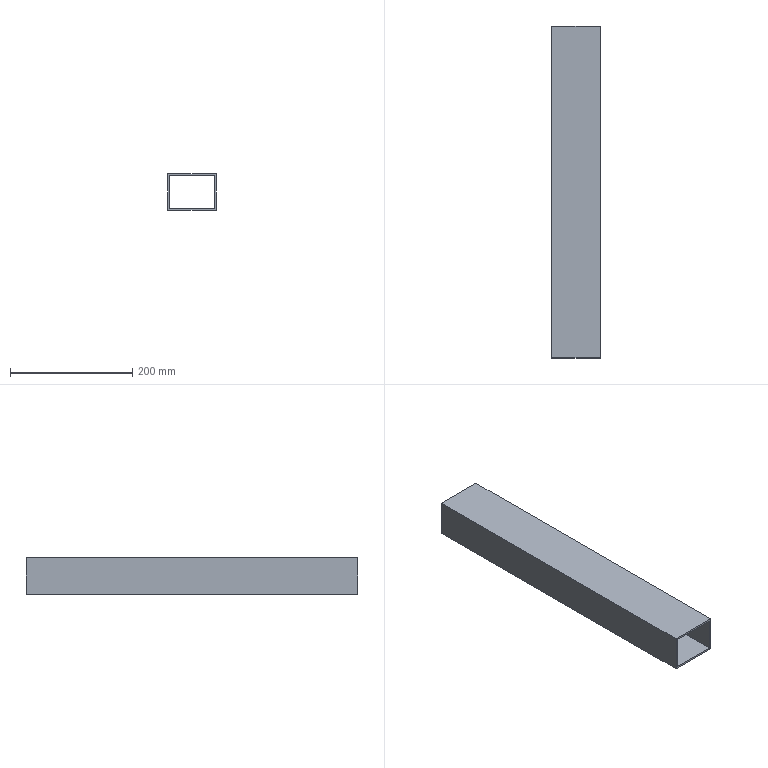Part | STEP file | Guide wheel mechanism revised.sldasm-Part-26 | 1 solid | 10 faces | box 80 x 541.99 x 60 mm | volume 435760 mm3 | plane 10
STEP:
#1=CARTESIAN_POINT('',(405.,1970.,445.));
#2=VERTEX_POINT('',#1);
#3=CARTESIAN_POINT('',(405.,1428.01,445.));
#4=VERTEX_POINT('',#3);
#5=CARTESIAN_POINT('',(405.,1970.,445.));
#6=DIRECTION('',(0.,-1.,0.));
#7=VECTOR('',#6,1000.);
#8=LINE('',#5,#7);
#9=EDGE_CURVE('',#2,#4,#8,.T.);
#10=ORIENTED_EDGE('',*,*,#9,.T.);
#11=CARTESIAN_POINT('',(405.,1428.01,505.));
#12=VERTEX_POINT('',#11);
#13=CARTESIAN_POINT('',(405.,1428.01,-160.471));
#14=DIRECTION('',(0.,0.,1.));
#15=VECTOR('',#14,1000.);
#16=LINE('',#13,#15);
#17=EDGE_CURVE('',#4,#12,#16,.T.);
#18=ORIENTED_EDGE('',*,*,#17,.T.);
#19=CARTESIAN_POINT('',(405.,1970.,505.));
#20=VERTEX_POINT('',#19);
#21=CARTESIAN_POINT('',(405.,1970.,505.));
#22=DIRECTION('',(0.,-1.,0.));
#23=VECTOR('',#22,1000.);
#24=LINE('',#21,#23);
#25=EDGE_CURVE('',#20,#12,#24,.T.);
#26=ORIENTED_EDGE('',*,*,#25,.F.);
#27=CARTESIAN_POINT('',(405.,1970.,505.));
#28=DIRECTION('',(0.,0.,1.));
#29=VECTOR('',#28,1000.);
#30=LINE('',#27,#29);
#31=EDGE_CURVE('',#2,#20,#30,.T.);
#32=ORIENTED_EDGE('',*,*,#31,.F.);
#33=EDGE_LOOP('',(#10,#18,#26,#32));
#34=FACE_OUTER_BOUND('',#33,.T.);
#35=CARTESIAN_POINT('',(405.,1970.,505.));
#36=DIRECTION('',(1.,0.,0.));
#37=DIRECTION('',(0.,0.,-1.));
#38=AXIS2_PLACEMENT_3D('',#35,#36,#37);
#39=PLANE('',#38);
#40=ADVANCED_FACE('',(#34),#39,.F.);
#41=ORIENTED_EDGE('',*,*,#25,.T.);
#42=CARTESIAN_POINT('',(485.,1428.01,505.));
#43=VERTEX_POINT('',#42);
#44=CARTESIAN_POINT('',(405.,1428.01,505.));
#45=DIRECTION('',(-1.,0.,0.));
#46=VECTOR('',#45,1000.);
#47=LINE('',#44,#46);
#48=EDGE_CURVE('',#43,#12,#47,.T.);
#49=ORIENTED_EDGE('',*,*,#48,.F.);
#50=CARTESIAN_POINT('',(485.,1970.,505.));
#51=VERTEX_POINT('',#50);
#52=CARTESIAN_POINT('',(485.,1970.,505.));
#53=DIRECTION('',(0.,-1.,0.));
#54=VECTOR('',#53,1000.);
#55=LINE('',#52,#54);
#56=EDGE_CURVE('',#51,#43,#55,.T.);
#57=ORIENTED_EDGE('',*,*,#56,.F.);
#58=CARTESIAN_POINT('',(485.,1970.,505.));
#59=DIRECTION('',(1.,0.,0.));
#60=VECTOR('',#59,1000.);
#61=LINE('',#58,#60);
#62=EDGE_CURVE('',#20,#51,#61,.T.);
#63=ORIENTED_EDGE('',*,*,#62,.F.);
#64=EDGE_LOOP('',(#41,#49,#57,#63));
#65=FACE_OUTER_BOUND('',#64,.T.);
#66=CARTESIAN_POINT('',(485.,1970.,505.));
#67=DIRECTION('',(0.,0.,-1.));
#68=DIRECTION('',(-1.,0.,0.));
#69=AXIS2_PLACEMENT_3D('',#66,#67,#68);
#70=PLANE('',#69);
#71=ADVANCED_FACE('',(#65),#70,.F.);
#72=ORIENTED_EDGE('',*,*,#56,.T.);
#73=CARTESIAN_POINT('',(485.,1428.01,445.));
#74=VERTEX_POINT('',#73);
#75=CARTESIAN_POINT('',(485.,1428.01,505.));
#76=DIRECTION('',(0.,0.,-1.));
#77=VECTOR('',#76,1000.);
#78=LINE('',#75,#77);
#79=EDGE_CURVE('',#43,#74,#78,.T.);
#80=ORIENTED_EDGE('',*,*,#79,.T.);
#81=CARTESIAN_POINT('',(485.,1970.,445.));
#82=VERTEX_POINT('',#81);
#83=CARTESIAN_POINT('',(485.,1970.,445.));
#84=DIRECTION('',(0.,-1.,0.));
#85=VECTOR('',#84,1000.);
#86=LINE('',#83,#85);
#87=EDGE_CURVE('',#82,#74,#86,.T.);
#88=ORIENTED_EDGE('',*,*,#87,.F.);
#89=CARTESIAN_POINT('',(485.,1970.,505.));
#90=DIRECTION('',(0.,0.,-1.));
#91=VECTOR('',#90,1000.);
#92=LINE('',#89,#91);
#93=EDGE_CURVE('',#51,#82,#92,.T.);
#94=ORIENTED_EDGE('',*,*,#93,.F.);
#95=EDGE_LOOP('',(#72,#80,#88,#94));
#96=FACE_OUTER_BOUND('',#95,.T.);
#97=CARTESIAN_POINT('',(485.,1970.,505.));
#98=DIRECTION('',(-1.,0.,0.));
#99=DIRECTION('',(0.,0.,1.));
#100=AXIS2_PLACEMENT_3D('',#97,#98,#99);
#101=PLANE('',#100);
#102=ADVANCED_FACE('',(#96),#101,.F.);
#103=ORIENTED_EDGE('',*,*,#87,.T.);
#104=CARTESIAN_POINT('',(405.,1428.01,445.));
#105=DIRECTION('',(1.,0.,0.));
#106=VECTOR('',#105,1000.);
#107=LINE('',#104,#106);
#108=EDGE_CURVE('',#4,#74,#107,.T.);
#109=ORIENTED_EDGE('',*,*,#108,.F.);
#110=ORIENTED_EDGE('',*,*,#9,.F.);
#111=CARTESIAN_POINT('',(485.,1970.,445.));
#112=DIRECTION('',(-1.,0.,0.));
#113=VECTOR('',#112,1000.);
#114=LINE('',#111,#113);
#115=EDGE_CURVE('',#82,#2,#114,.T.);
#116=ORIENTED_EDGE('',*,*,#115,.F.);
#117=EDGE_LOOP('',(#103,#109,#110,#116));
#118=FACE_OUTER_BOUND('',#117,.T.);
#119=CARTESIAN_POINT('',(485.,1970.,445.));
#120=DIRECTION('',(0.,0.,1.));
#121=DIRECTION('',(1.,0.,0.));
#122=AXIS2_PLACEMENT_3D('',#119,#120,#121);
#123=PLANE('',#122);
#124=ADVANCED_FACE('',(#118),#123,.F.);
#125=CARTESIAN_POINT('',(482.,1428.01,502.));
#126=VERTEX_POINT('',#125);
#127=CARTESIAN_POINT('',(482.,1428.01,448.));
#128=VERTEX_POINT('',#127);
#129=CARTESIAN_POINT('',(482.,1428.01,502.));
#130=DIRECTION('',(0.,0.,-1.));
#131=VECTOR('',#130,1000.);
#132=LINE('',#129,#131);
#133=EDGE_CURVE('',#126,#128,#132,.T.);
#134=ORIENTED_EDGE('',*,*,#133,.F.);
#135=CARTESIAN_POINT('',(482.,1970.,502.));
#136=VERTEX_POINT('',#135);
#137=CARTESIAN_POINT('',(482.,1970.,502.));
#138=DIRECTION('',(0.,-1.,0.));
#139=VECTOR('',#138,1000.);
#140=LINE('',#137,#139);
#141=EDGE_CURVE('',#136,#126,#140,.T.);
#142=ORIENTED_EDGE('',*,*,#141,.F.);
#143=CARTESIAN_POINT('',(482.,1970.,448.));
#144=VERTEX_POINT('',#143);
#145=CARTESIAN_POINT('',(482.,1970.,502.));
#146=DIRECTION('',(0.,0.,-1.));
#147=VECTOR('',#146,1000.);
#148=LINE('',#145,#147);
#149=EDGE_CURVE('',#136,#144,#148,.T.);
#150=ORIENTED_EDGE('',*,*,#149,.T.);
#151=CARTESIAN_POINT('',(482.,1970.,448.));
#152=DIRECTION('',(0.,-1.,0.));
#153=VECTOR('',#152,1000.);
#154=LINE('',#151,#153);
#155=EDGE_CURVE('',#144,#128,#154,.T.);
#156=ORIENTED_EDGE('',*,*,#155,.T.);
#157=EDGE_LOOP('',(#134,#142,#150,#156));
#158=FACE_OUTER_BOUND('',#157,.T.);
#159=CARTESIAN_POINT('',(482.,1970.,502.));
#160=DIRECTION('',(-1.,0.,0.));
#161=DIRECTION('',(0.,0.,1.));
#162=AXIS2_PLACEMENT_3D('',#159,#160,#161);
#163=PLANE('',#162);
#164=ADVANCED_FACE('',(#158),#163,.T.);
#165=CARTESIAN_POINT('',(408.,1428.01,448.));
#166=VERTEX_POINT('',#165);
#167=CARTESIAN_POINT('',(482.,1428.01,448.));
#168=DIRECTION('',(-1.,0.,0.));
#169=VECTOR('',#168,1000.);
#170=LINE('',#167,#169);
#171=EDGE_CURVE('',#128,#166,#170,.T.);
#172=ORIENTED_EDGE('',*,*,#171,.F.);
#173=ORIENTED_EDGE('',*,*,#155,.F.);
#174=CARTESIAN_POINT('',(408.,1970.,448.));
#175=VERTEX_POINT('',#174);
#176=CARTESIAN_POINT('',(482.,1970.,448.));
#177=DIRECTION('',(-1.,0.,0.));
#178=VECTOR('',#177,1000.);
#179=LINE('',#176,#178);
#180=EDGE_CURVE('',#144,#175,#179,.T.);
#181=ORIENTED_EDGE('',*,*,#180,.T.);
#182=CARTESIAN_POINT('',(408.,1970.,448.));
#183=DIRECTION('',(0.,-1.,0.));
#184=VECTOR('',#183,1000.);
#185=LINE('',#182,#184);
#186=EDGE_CURVE('',#175,#166,#185,.T.);
#187=ORIENTED_EDGE('',*,*,#186,.T.);
#188=EDGE_LOOP('',(#172,#173,#181,#187));
#189=FACE_OUTER_BOUND('',#188,.T.);
#190=CARTESIAN_POINT('',(482.,1970.,448.));
#191=DIRECTION('',(0.,0.,1.));
#192=DIRECTION('',(1.,0.,0.));
#193=AXIS2_PLACEMENT_3D('',#190,#191,#192);
#194=PLANE('',#193);
#195=ADVANCED_FACE('',(#189),#194,.T.);
#196=CARTESIAN_POINT('',(408.,1428.01,502.));
#197=VERTEX_POINT('',#196);
#198=CARTESIAN_POINT('',(408.,1428.01,502.));
#199=DIRECTION('',(0.,0.,1.));
#200=VECTOR('',#199,1000.);
#201=LINE('',#198,#200);
#202=EDGE_CURVE('',#166,#197,#201,.T.);
#203=ORIENTED_EDGE('',*,*,#202,.F.);
#204=ORIENTED_EDGE('',*,*,#186,.F.);
#205=CARTESIAN_POINT('',(408.,1970.,502.));
#206=VERTEX_POINT('',#205);
#207=CARTESIAN_POINT('',(408.,1970.,502.));
#208=DIRECTION('',(0.,0.,1.));
#209=VECTOR('',#208,1000.);
#210=LINE('',#207,#209);
#211=EDGE_CURVE('',#175,#206,#210,.T.);
#212=ORIENTED_EDGE('',*,*,#211,.T.);
#213=CARTESIAN_POINT('',(408.,1970.,502.));
#214=DIRECTION('',(0.,-1.,0.));
#215=VECTOR('',#214,1000.);
#216=LINE('',#213,#215);
#217=EDGE_CURVE('',#206,#197,#216,.T.);
#218=ORIENTED_EDGE('',*,*,#217,.T.);
#219=EDGE_LOOP('',(#203,#204,#212,#218));
#220=FACE_OUTER_BOUND('',#219,.T.);
#221=CARTESIAN_POINT('',(408.,1970.,502.));
#222=DIRECTION('',(1.,0.,0.));
#223=DIRECTION('',(0.,0.,-1.));
#224=AXIS2_PLACEMENT_3D('',#221,#222,#223);
#225=PLANE('',#224);
#226=ADVANCED_FACE('',(#220),#225,.T.);
#227=CARTESIAN_POINT('',(482.,1428.01,502.));
#228=DIRECTION('',(1.,0.,0.));
#229=VECTOR('',#228,1000.);
#230=LINE('',#227,#229);
#231=EDGE_CURVE('',#197,#126,#230,.T.);
#232=ORIENTED_EDGE('',*,*,#231,.F.);
#233=ORIENTED_EDGE('',*,*,#217,.F.);
#234=CARTESIAN_POINT('',(482.,1970.,502.));
#235=DIRECTION('',(1.,0.,0.));
#236=VECTOR('',#235,1000.);
#237=LINE('',#234,#236);
#238=EDGE_CURVE('',#206,#136,#237,.T.);
#239=ORIENTED_EDGE('',*,*,#238,.T.);
#240=ORIENTED_EDGE('',*,*,#141,.T.);
#241=EDGE_LOOP('',(#232,#233,#239,#240));
#242=FACE_OUTER_BOUND('',#241,.T.);
#243=CARTESIAN_POINT('',(482.,1970.,502.));
#244=DIRECTION('',(0.,0.,-1.));
#245=DIRECTION('',(-1.,0.,0.));
#246=AXIS2_PLACEMENT_3D('',#243,#244,#245);
#247=PLANE('',#246);
#248=ADVANCED_FACE('',(#242),#247,.T.);
#249=ORIENTED_EDGE('',*,*,#31,.T.);
#250=ORIENTED_EDGE('',*,*,#62,.T.);
#251=ORIENTED_EDGE('',*,*,#93,.T.);
#252=ORIENTED_EDGE('',*,*,#115,.T.);
#253=EDGE_LOOP('',(#249,#250,#251,#252));
#254=FACE_OUTER_BOUND('',#253,.T.);
#255=ORIENTED_EDGE('',*,*,#180,.F.);
#256=ORIENTED_EDGE('',*,*,#149,.F.);
#257=ORIENTED_EDGE('',*,*,#238,.F.);
#258=ORIENTED_EDGE('',*,*,#211,.F.);
#259=EDGE_LOOP('',(#255,#256,#257,#258));
#260=FACE_BOUND('',#259,.T.);
#261=CARTESIAN_POINT('',(0.,1970.,0.));
#262=DIRECTION('',(0.,1.,0.));
#263=DIRECTION('',(0.,0.,1.));
#264=AXIS2_PLACEMENT_3D('',#261,#262,#263);
#265=PLANE('',#264);
#266=ADVANCED_FACE('',(#254,#260),#265,.T.);
#267=ORIENTED_EDGE('',*,*,#133,.T.);
#268=ORIENTED_EDGE('',*,*,#171,.T.);
#269=ORIENTED_EDGE('',*,*,#202,.T.);
#270=ORIENTED_EDGE('',*,*,#231,.T.);
#271=EDGE_LOOP('',(#267,#268,#269,#270));
#272=FACE_BOUND('',#271,.T.);
#273=ORIENTED_EDGE('',*,*,#48,.T.);
#274=ORIENTED_EDGE('',*,*,#17,.F.);
#275=ORIENTED_EDGE('',*,*,#108,.T.);
#276=ORIENTED_EDGE('',*,*,#79,.F.);
#277=EDGE_LOOP('',(#273,#274,#275,#276));
#278=FACE_OUTER_BOUND('',#277,.T.);
#279=CARTESIAN_POINT('',(405.,1428.01,-160.471));
#280=DIRECTION('',(0.,1.,0.));
#281=DIRECTION('',(0.,0.,1.));
#282=AXIS2_PLACEMENT_3D('',#279,#280,#281);
#283=PLANE('',#282);
#284=ADVANCED_FACE('',(#272,#278),#283,.F.);
#285=CLOSED_SHELL('',(#40,#71,#102,#124,#164,#195,#226,#248,#266,#284));
#286=MANIFOLD_SOLID_BREP('',#285);
#287=CARTESIAN_POINT('',(0.,0.,0.));
#288=DIRECTION('',(0.,0.,1.));
#289=DIRECTION('',(1.,0.,0.));
#290=AXIS2_PLACEMENT_3D('',#287,#288,#289);
#291=(LENGTH_UNIT()NAMED_UNIT(*)SI_UNIT(.MILLI.,.METRE.));
#292=UNCERTAINTY_MEASURE_WITH_UNIT(LENGTH_MEASURE(0.00001),#291,'','');
#293=(NAMED_UNIT(*)PLANE_ANGLE_UNIT()SI_UNIT($,.RADIAN.));
#294=(NAMED_UNIT(*)SI_UNIT($,.STERADIAN.)SOLID_ANGLE_UNIT());
#295=(GEOMETRIC_REPRESENTATION_CONTEXT(3)GLOBAL_UNCERTAINTY_ASSIGNED_CONTEXT((#292))GLOBAL_UNIT_ASSIGNED_CONTEXT((#291,#293,#294))REPRESENTATION_CONTEXT('',''));
#296=ADVANCED_BREP_SHAPE_REPRESENTATION('',(#286,#290),#295);